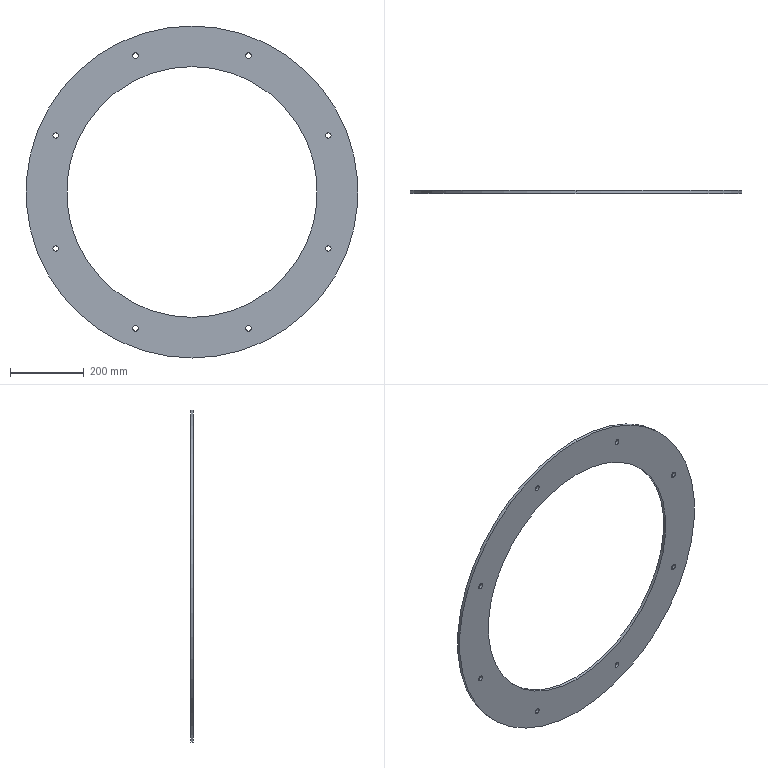Part | SolidWorks | features Extrusion 1, HoleWzd 1 | 1 solid | 22 faces | box 900 x 8 x 900 mm | volume 2172725 mm3 | cylinder 20 | plane 2 | commonest cylinder face diameters 15 x16 680 x2 900 x2
STEP:
#1=CARTESIAN_POINT('',(153.073,-4.,-377.052));
#2=VERTEX_POINT('',#1);
#3=CARTESIAN_POINT('',(153.073,-4.,-362.052));
#4=VERTEX_POINT('',#3);
#5=CARTESIAN_POINT('',(153.073,-4.,-369.552));
#6=DIRECTION('',(0.,1.,0.));
#7=DIRECTION('',(0.,0.,1.));
#8=AXIS2_PLACEMENT_3D('',#5,#6,#7);
#9=CIRCLE('',#8,7.5);
#10=EDGE_CURVE('',#2,#4,#9,.T.);
#11=ORIENTED_EDGE('',*,*,#10,.F.);
#12=CARTESIAN_POINT('',(153.073,4.,-377.052));
#13=VERTEX_POINT('',#12);
#14=CARTESIAN_POINT('',(153.073,4.,-377.052));
#15=DIRECTION('',(0.,1.,0.));
#16=VECTOR('',#15,1000.);
#17=LINE('',#14,#16);
#18=EDGE_CURVE('',#2,#13,#17,.T.);
#19=ORIENTED_EDGE('',*,*,#18,.T.);
#20=CARTESIAN_POINT('',(153.073,4.,-362.052));
#21=VERTEX_POINT('',#20);
#22=CARTESIAN_POINT('',(153.073,4.,-369.552));
#23=DIRECTION('',(0.,1.,0.));
#24=DIRECTION('',(0.,0.,1.));
#25=AXIS2_PLACEMENT_3D('',#22,#23,#24);
#26=CIRCLE('',#25,7.5);
#27=EDGE_CURVE('',#13,#21,#26,.T.);
#28=ORIENTED_EDGE('',*,*,#27,.T.);
#29=CARTESIAN_POINT('',(153.073,4.,-362.052));
#30=DIRECTION('',(0.,1.,0.));
#31=VECTOR('',#30,1000.);
#32=LINE('',#29,#31);
#33=EDGE_CURVE('',#4,#21,#32,.T.);
#34=ORIENTED_EDGE('',*,*,#33,.F.);
#35=EDGE_LOOP('',(#11,#19,#28,#34));
#36=FACE_OUTER_BOUND('',#35,.T.);
#37=CARTESIAN_POINT('',(153.073,4.,-369.552));
#38=DIRECTION('',(0.,1.,0.));
#39=DIRECTION('',(0.,0.,1.));
#40=AXIS2_PLACEMENT_3D('',#37,#38,#39);
#41=CYLINDRICAL_SURFACE('',#40,7.5);
#42=ADVANCED_FACE('',(#36),#41,.F.);
#43=CARTESIAN_POINT('',(369.552,-4.,-160.573));
#44=VERTEX_POINT('',#43);
#45=CARTESIAN_POINT('',(369.552,-4.,-145.573));
#46=VERTEX_POINT('',#45);
#47=CARTESIAN_POINT('',(369.552,-4.,-153.073));
#48=DIRECTION('',(0.,1.,0.));
#49=DIRECTION('',(0.,0.,1.));
#50=AXIS2_PLACEMENT_3D('',#47,#48,#49);
#51=CIRCLE('',#50,7.5);
#52=EDGE_CURVE('',#44,#46,#51,.T.);
#53=ORIENTED_EDGE('',*,*,#52,.F.);
#54=CARTESIAN_POINT('',(369.552,4.,-160.573));
#55=VERTEX_POINT('',#54);
#56=CARTESIAN_POINT('',(369.552,4.,-160.573));
#57=DIRECTION('',(0.,1.,0.));
#58=VECTOR('',#57,1000.);
#59=LINE('',#56,#58);
#60=EDGE_CURVE('',#44,#55,#59,.T.);
#61=ORIENTED_EDGE('',*,*,#60,.T.);
#62=CARTESIAN_POINT('',(369.552,4.,-145.573));
#63=VERTEX_POINT('',#62);
#64=CARTESIAN_POINT('',(369.552,4.,-153.073));
#65=DIRECTION('',(0.,1.,0.));
#66=DIRECTION('',(0.,0.,1.));
#67=AXIS2_PLACEMENT_3D('',#64,#65,#66);
#68=CIRCLE('',#67,7.5);
#69=EDGE_CURVE('',#55,#63,#68,.T.);
#70=ORIENTED_EDGE('',*,*,#69,.T.);
#71=CARTESIAN_POINT('',(369.552,4.,-145.573));
#72=DIRECTION('',(0.,1.,0.));
#73=VECTOR('',#72,1000.);
#74=LINE('',#71,#73);
#75=EDGE_CURVE('',#46,#63,#74,.T.);
#76=ORIENTED_EDGE('',*,*,#75,.F.);
#77=EDGE_LOOP('',(#53,#61,#70,#76));
#78=FACE_OUTER_BOUND('',#77,.T.);
#79=CARTESIAN_POINT('',(369.552,4.,-153.073));
#80=DIRECTION('',(0.,1.,0.));
#81=DIRECTION('',(0.,0.,1.));
#82=AXIS2_PLACEMENT_3D('',#79,#80,#81);
#83=CYLINDRICAL_SURFACE('',#82,7.5);
#84=ADVANCED_FACE('',(#78),#83,.F.);
#85=CARTESIAN_POINT('',(369.552,-4.,145.573));
#86=VERTEX_POINT('',#85);
#87=CARTESIAN_POINT('',(369.552,-4.,160.573));
#88=VERTEX_POINT('',#87);
#89=CARTESIAN_POINT('',(369.552,-4.,153.073));
#90=DIRECTION('',(0.,1.,0.));
#91=DIRECTION('',(0.,0.,1.));
#92=AXIS2_PLACEMENT_3D('',#89,#90,#91);
#93=CIRCLE('',#92,7.5);
#94=EDGE_CURVE('',#86,#88,#93,.T.);
#95=ORIENTED_EDGE('',*,*,#94,.F.);
#96=CARTESIAN_POINT('',(369.552,4.,145.573));
#97=VERTEX_POINT('',#96);
#98=CARTESIAN_POINT('',(369.552,4.,145.573));
#99=DIRECTION('',(0.,1.,0.));
#100=VECTOR('',#99,1000.);
#101=LINE('',#98,#100);
#102=EDGE_CURVE('',#86,#97,#101,.T.);
#103=ORIENTED_EDGE('',*,*,#102,.T.);
#104=CARTESIAN_POINT('',(369.552,4.,160.573));
#105=VERTEX_POINT('',#104);
#106=CARTESIAN_POINT('',(369.552,4.,153.073));
#107=DIRECTION('',(0.,1.,0.));
#108=DIRECTION('',(0.,0.,1.));
#109=AXIS2_PLACEMENT_3D('',#106,#107,#108);
#110=CIRCLE('',#109,7.5);
#111=EDGE_CURVE('',#97,#105,#110,.T.);
#112=ORIENTED_EDGE('',*,*,#111,.T.);
#113=CARTESIAN_POINT('',(369.552,4.,160.573));
#114=DIRECTION('',(0.,1.,0.));
#115=VECTOR('',#114,1000.);
#116=LINE('',#113,#115);
#117=EDGE_CURVE('',#88,#105,#116,.T.);
#118=ORIENTED_EDGE('',*,*,#117,.F.);
#119=EDGE_LOOP('',(#95,#103,#112,#118));
#120=FACE_OUTER_BOUND('',#119,.T.);
#121=CARTESIAN_POINT('',(369.552,4.,153.073));
#122=DIRECTION('',(0.,1.,0.));
#123=DIRECTION('',(0.,0.,1.));
#124=AXIS2_PLACEMENT_3D('',#121,#122,#123);
#125=CYLINDRICAL_SURFACE('',#124,7.5);
#126=ADVANCED_FACE('',(#120),#125,.F.);
#127=CARTESIAN_POINT('',(153.073,-4.,362.052));
#128=VERTEX_POINT('',#127);
#129=CARTESIAN_POINT('',(153.073,-4.,377.052));
#130=VERTEX_POINT('',#129);
#131=CARTESIAN_POINT('',(153.073,-4.,369.552));
#132=DIRECTION('',(0.,1.,0.));
#133=DIRECTION('',(0.,0.,1.));
#134=AXIS2_PLACEMENT_3D('',#131,#132,#133);
#135=CIRCLE('',#134,7.5);
#136=EDGE_CURVE('',#128,#130,#135,.T.);
#137=ORIENTED_EDGE('',*,*,#136,.F.);
#138=CARTESIAN_POINT('',(153.073,4.,362.052));
#139=VERTEX_POINT('',#138);
#140=CARTESIAN_POINT('',(153.073,4.,362.052));
#141=DIRECTION('',(0.,1.,0.));
#142=VECTOR('',#141,1000.);
#143=LINE('',#140,#142);
#144=EDGE_CURVE('',#128,#139,#143,.T.);
#145=ORIENTED_EDGE('',*,*,#144,.T.);
#146=CARTESIAN_POINT('',(153.073,4.,377.052));
#147=VERTEX_POINT('',#146);
#148=CARTESIAN_POINT('',(153.073,4.,369.552));
#149=DIRECTION('',(0.,1.,0.));
#150=DIRECTION('',(0.,0.,1.));
#151=AXIS2_PLACEMENT_3D('',#148,#149,#150);
#152=CIRCLE('',#151,7.5);
#153=EDGE_CURVE('',#139,#147,#152,.T.);
#154=ORIENTED_EDGE('',*,*,#153,.T.);
#155=CARTESIAN_POINT('',(153.073,4.,377.052));
#156=DIRECTION('',(0.,1.,0.));
#157=VECTOR('',#156,1000.);
#158=LINE('',#155,#157);
#159=EDGE_CURVE('',#130,#147,#158,.T.);
#160=ORIENTED_EDGE('',*,*,#159,.F.);
#161=EDGE_LOOP('',(#137,#145,#154,#160));
#162=FACE_OUTER_BOUND('',#161,.T.);
#163=CARTESIAN_POINT('',(153.073,4.,369.552));
#164=DIRECTION('',(0.,1.,0.));
#165=DIRECTION('',(0.,0.,1.));
#166=AXIS2_PLACEMENT_3D('',#163,#164,#165);
#167=CYLINDRICAL_SURFACE('',#166,7.5);
#168=ADVANCED_FACE('',(#162),#167,.F.);
#169=CARTESIAN_POINT('',(-153.073,-4.,362.052));
#170=VERTEX_POINT('',#169);
#171=CARTESIAN_POINT('',(-153.073,-4.,377.052));
#172=VERTEX_POINT('',#171);
#173=CARTESIAN_POINT('',(-153.073,-4.,369.552));
#174=DIRECTION('',(0.,1.,0.));
#175=DIRECTION('',(0.,0.,1.));
#176=AXIS2_PLACEMENT_3D('',#173,#174,#175);
#177=CIRCLE('',#176,7.5);
#178=EDGE_CURVE('',#170,#172,#177,.T.);
#179=ORIENTED_EDGE('',*,*,#178,.F.);
#180=CARTESIAN_POINT('',(-153.073,4.,362.052));
#181=VERTEX_POINT('',#180);
#182=CARTESIAN_POINT('',(-153.073,4.,362.052));
#183=DIRECTION('',(0.,1.,0.));
#184=VECTOR('',#183,1000.);
#185=LINE('',#182,#184);
#186=EDGE_CURVE('',#170,#181,#185,.T.);
#187=ORIENTED_EDGE('',*,*,#186,.T.);
#188=CARTESIAN_POINT('',(-153.073,4.,377.052));
#189=VERTEX_POINT('',#188);
#190=CARTESIAN_POINT('',(-153.073,4.,369.552));
#191=DIRECTION('',(0.,1.,0.));
#192=DIRECTION('',(0.,0.,1.));
#193=AXIS2_PLACEMENT_3D('',#190,#191,#192);
#194=CIRCLE('',#193,7.5);
#195=EDGE_CURVE('',#181,#189,#194,.T.);
#196=ORIENTED_EDGE('',*,*,#195,.T.);
#197=CARTESIAN_POINT('',(-153.073,4.,377.052));
#198=DIRECTION('',(0.,1.,0.));
#199=VECTOR('',#198,1000.);
#200=LINE('',#197,#199);
#201=EDGE_CURVE('',#172,#189,#200,.T.);
#202=ORIENTED_EDGE('',*,*,#201,.F.);
#203=EDGE_LOOP('',(#179,#187,#196,#202));
#204=FACE_OUTER_BOUND('',#203,.T.);
#205=CARTESIAN_POINT('',(-153.073,4.,369.552));
#206=DIRECTION('',(0.,1.,0.));
#207=DIRECTION('',(0.,0.,1.));
#208=AXIS2_PLACEMENT_3D('',#205,#206,#207);
#209=CYLINDRICAL_SURFACE('',#208,7.5);
#210=ADVANCED_FACE('',(#204),#209,.F.);
#211=CARTESIAN_POINT('',(-369.552,-4.,145.573));
#212=VERTEX_POINT('',#211);
#213=CARTESIAN_POINT('',(-369.552,-4.,160.573));
#214=VERTEX_POINT('',#213);
#215=CARTESIAN_POINT('',(-369.552,-4.,153.073));
#216=DIRECTION('',(0.,1.,0.));
#217=DIRECTION('',(0.,0.,1.));
#218=AXIS2_PLACEMENT_3D('',#215,#216,#217);
#219=CIRCLE('',#218,7.5);
#220=EDGE_CURVE('',#212,#214,#219,.T.);
#221=ORIENTED_EDGE('',*,*,#220,.F.);
#222=CARTESIAN_POINT('',(-369.552,4.,145.573));
#223=VERTEX_POINT('',#222);
#224=CARTESIAN_POINT('',(-369.552,4.,145.573));
#225=DIRECTION('',(0.,1.,0.));
#226=VECTOR('',#225,1000.);
#227=LINE('',#224,#226);
#228=EDGE_CURVE('',#212,#223,#227,.T.);
#229=ORIENTED_EDGE('',*,*,#228,.T.);
#230=CARTESIAN_POINT('',(-369.552,4.,160.573));
#231=VERTEX_POINT('',#230);
#232=CARTESIAN_POINT('',(-369.552,4.,153.073));
#233=DIRECTION('',(0.,1.,0.));
#234=DIRECTION('',(0.,0.,1.));
#235=AXIS2_PLACEMENT_3D('',#232,#233,#234);
#236=CIRCLE('',#235,7.5);
#237=EDGE_CURVE('',#223,#231,#236,.T.);
#238=ORIENTED_EDGE('',*,*,#237,.T.);
#239=CARTESIAN_POINT('',(-369.552,4.,160.573));
#240=DIRECTION('',(0.,1.,0.));
#241=VECTOR('',#240,1000.);
#242=LINE('',#239,#241);
#243=EDGE_CURVE('',#214,#231,#242,.T.);
#244=ORIENTED_EDGE('',*,*,#243,.F.);
#245=EDGE_LOOP('',(#221,#229,#238,#244));
#246=FACE_OUTER_BOUND('',#245,.T.);
#247=CARTESIAN_POINT('',(-369.552,4.,153.073));
#248=DIRECTION('',(0.,1.,0.));
#249=DIRECTION('',(0.,0.,1.));
#250=AXIS2_PLACEMENT_3D('',#247,#248,#249);
#251=CYLINDRICAL_SURFACE('',#250,7.5);
#252=ADVANCED_FACE('',(#246),#251,.F.);
#253=CARTESIAN_POINT('',(-369.552,-4.,-160.573));
#254=VERTEX_POINT('',#253);
#255=CARTESIAN_POINT('',(-369.552,-4.,-145.573));
#256=VERTEX_POINT('',#255);
#257=CARTESIAN_POINT('',(-369.552,-4.,-153.073));
#258=DIRECTION('',(0.,1.,0.));
#259=DIRECTION('',(0.,0.,1.));
#260=AXIS2_PLACEMENT_3D('',#257,#258,#259);
#261=CIRCLE('',#260,7.5);
#262=EDGE_CURVE('',#254,#256,#261,.T.);
#263=ORIENTED_EDGE('',*,*,#262,.F.);
#264=CARTESIAN_POINT('',(-369.552,4.,-160.573));
#265=VERTEX_POINT('',#264);
#266=CARTESIAN_POINT('',(-369.552,4.,-160.573));
#267=DIRECTION('',(0.,1.,0.));
#268=VECTOR('',#267,1000.);
#269=LINE('',#266,#268);
#270=EDGE_CURVE('',#254,#265,#269,.T.);
#271=ORIENTED_EDGE('',*,*,#270,.T.);
#272=CARTESIAN_POINT('',(-369.552,4.,-145.573));
#273=VERTEX_POINT('',#272);
#274=CARTESIAN_POINT('',(-369.552,4.,-153.073));
#275=DIRECTION('',(0.,1.,0.));
#276=DIRECTION('',(0.,0.,1.));
#277=AXIS2_PLACEMENT_3D('',#274,#275,#276);
#278=CIRCLE('',#277,7.5);
#279=EDGE_CURVE('',#265,#273,#278,.T.);
#280=ORIENTED_EDGE('',*,*,#279,.T.);
#281=CARTESIAN_POINT('',(-369.552,4.,-145.573));
#282=DIRECTION('',(0.,1.,0.));
#283=VECTOR('',#282,1000.);
#284=LINE('',#281,#283);
#285=EDGE_CURVE('',#256,#273,#284,.T.);
#286=ORIENTED_EDGE('',*,*,#285,.F.);
#287=EDGE_LOOP('',(#263,#271,#280,#286));
#288=FACE_OUTER_BOUND('',#287,.T.);
#289=CARTESIAN_POINT('',(-369.552,4.,-153.073));
#290=DIRECTION('',(0.,1.,0.));
#291=DIRECTION('',(0.,0.,1.));
#292=AXIS2_PLACEMENT_3D('',#289,#290,#291);
#293=CYLINDRICAL_SURFACE('',#292,7.5);
#294=ADVANCED_FACE('',(#288),#293,.F.);
#295=CARTESIAN_POINT('',(-153.073,-4.,-377.052));
#296=VERTEX_POINT('',#295);
#297=CARTESIAN_POINT('',(-153.073,-4.,-362.052));
#298=VERTEX_POINT('',#297);
#299=CARTESIAN_POINT('',(-153.073,-4.,-369.552));
#300=DIRECTION('',(0.,1.,0.));
#301=DIRECTION('',(0.,0.,1.));
#302=AXIS2_PLACEMENT_3D('',#299,#300,#301);
#303=CIRCLE('',#302,7.5);
#304=EDGE_CURVE('',#296,#298,#303,.T.);
#305=ORIENTED_EDGE('',*,*,#304,.F.);
#306=CARTESIAN_POINT('',(-153.073,4.,-377.052));
#307=VERTEX_POINT('',#306);
#308=CARTESIAN_POINT('',(-153.073,4.,-377.052));
#309=DIRECTION('',(0.,1.,0.));
#310=VECTOR('',#309,1000.);
#311=LINE('',#308,#310);
#312=EDGE_CURVE('',#296,#307,#311,.T.);
#313=ORIENTED_EDGE('',*,*,#312,.T.);
#314=CARTESIAN_POINT('',(-153.073,4.,-362.052));
#315=VERTEX_POINT('',#314);
#316=CARTESIAN_POINT('',(-153.073,4.,-369.552));
#317=DIRECTION('',(0.,1.,0.));
#318=DIRECTION('',(0.,0.,1.));
#319=AXIS2_PLACEMENT_3D('',#316,#317,#318);
#320=CIRCLE('',#319,7.5);
#321=EDGE_CURVE('',#307,#315,#320,.T.);
#322=ORIENTED_EDGE('',*,*,#321,.T.);
#323=CARTESIAN_POINT('',(-153.073,4.,-362.052));
#324=DIRECTION('',(0.,1.,0.));
#325=VECTOR('',#324,1000.);
#326=LINE('',#323,#325);
#327=EDGE_CURVE('',#298,#315,#326,.T.);
#328=ORIENTED_EDGE('',*,*,#327,.F.);
#329=EDGE_LOOP('',(#305,#313,#322,#328));
#330=FACE_OUTER_BOUND('',#329,.T.);
#331=CARTESIAN_POINT('',(-153.073,4.,-369.552));
#332=DIRECTION('',(0.,1.,0.));
#333=DIRECTION('',(0.,0.,1.));
#334=AXIS2_PLACEMENT_3D('',#331,#332,#333);
#335=CYLINDRICAL_SURFACE('',#334,7.5);
#336=ADVANCED_FACE('',(#330),#335,.F.);
#337=CARTESIAN_POINT('',(0.,4.,-340.));
#338=VERTEX_POINT('',#337);
#339=CARTESIAN_POINT('',(0.,4.,340.));
#340=VERTEX_POINT('',#339);
#341=CARTESIAN_POINT('',(0.,4.,0.));
#342=DIRECTION('',(0.,1.,0.));
#343=DIRECTION('',(0.,0.,1.));
#344=AXIS2_PLACEMENT_3D('',#341,#342,#343);
#345=CIRCLE('',#344,340.);
#346=EDGE_CURVE('',#338,#340,#345,.T.);
#347=ORIENTED_EDGE('',*,*,#346,.T.);
#348=CARTESIAN_POINT('',(0.,-4.,340.));
#349=VERTEX_POINT('',#348);
#350=CARTESIAN_POINT('',(0.,4.,340.));
#351=DIRECTION('',(0.,-1.,0.));
#352=VECTOR('',#351,1000.);
#353=LINE('',#350,#352);
#354=EDGE_CURVE('',#340,#349,#353,.T.);
#355=ORIENTED_EDGE('',*,*,#354,.T.);
#356=CARTESIAN_POINT('',(0.,-4.,-340.));
#357=VERTEX_POINT('',#356);
#358=CARTESIAN_POINT('',(0.,-4.,0.));
#359=DIRECTION('',(0.,1.,0.));
#360=DIRECTION('',(0.,0.,1.));
#361=AXIS2_PLACEMENT_3D('',#358,#359,#360);
#362=CIRCLE('',#361,340.);
#363=EDGE_CURVE('',#357,#349,#362,.T.);
#364=ORIENTED_EDGE('',*,*,#363,.F.);
#365=CARTESIAN_POINT('',(0.,4.,-340.));
#366=DIRECTION('',(0.,-1.,0.));
#367=VECTOR('',#366,1000.);
#368=LINE('',#365,#367);
#369=EDGE_CURVE('',#338,#357,#368,.T.);
#370=ORIENTED_EDGE('',*,*,#369,.F.);
#371=EDGE_LOOP('',(#347,#355,#364,#370));
#372=FACE_OUTER_BOUND('',#371,.T.);
#373=CARTESIAN_POINT('',(0.,4.,0.));
#374=DIRECTION('',(0.,-1.,0.));
#375=DIRECTION('',(0.,0.,-1.));
#376=AXIS2_PLACEMENT_3D('',#373,#374,#375);
#377=CYLINDRICAL_SURFACE('',#376,340.);
#378=ADVANCED_FACE('',(#372),#377,.F.);
#379=CARTESIAN_POINT('',(0.,4.,450.));
#380=VERTEX_POINT('',#379);
#381=CARTESIAN_POINT('',(0.,4.,-450.));
#382=VERTEX_POINT('',#381);
#383=CARTESIAN_POINT('',(0.,4.,0.));
#384=DIRECTION('',(0.,1.,0.));
#385=DIRECTION('',(0.,0.,1.));
#386=AXIS2_PLACEMENT_3D('',#383,#384,#385);
#387=CIRCLE('',#386,450.);
#388=EDGE_CURVE('',#380,#382,#387,.T.);
#389=ORIENTED_EDGE('',*,*,#388,.F.);
#390=CARTESIAN_POINT('',(0.,-4.,450.));
#391=VERTEX_POINT('',#390);
#392=CARTESIAN_POINT('',(0.,4.,450.));
#393=DIRECTION('',(0.,-1.,0.));
#394=VECTOR('',#393,1000.);
#395=LINE('',#392,#394);
#396=EDGE_CURVE('',#380,#391,#395,.T.);
#397=ORIENTED_EDGE('',*,*,#396,.T.);
#398=CARTESIAN_POINT('',(0.,-4.,-450.));
#399=VERTEX_POINT('',#398);
#400=CARTESIAN_POINT('',(0.,-4.,0.));
#401=DIRECTION('',(0.,1.,0.));
#402=DIRECTION('',(0.,0.,1.));
#403=AXIS2_PLACEMENT_3D('',#400,#401,#402);
#404=CIRCLE('',#403,450.);
#405=EDGE_CURVE('',#391,#399,#404,.T.);
#406=ORIENTED_EDGE('',*,*,#405,.T.);
#407=CARTESIAN_POINT('',(0.,4.,-450.));
#408=DIRECTION('',(0.,-1.,0.));
#409=VECTOR('',#408,1000.);
#410=LINE('',#407,#409);
#411=EDGE_CURVE('',#382,#399,#410,.T.);
#412=ORIENTED_EDGE('',*,*,#411,.F.);
#413=EDGE_LOOP('',(#389,#397,#406,#412));
#414=FACE_OUTER_BOUND('',#413,.T.);
#415=CARTESIAN_POINT('',(0.,4.,0.));
#416=DIRECTION('',(0.,-1.,0.));
#417=DIRECTION('',(0.,0.,-1.));
#418=AXIS2_PLACEMENT_3D('',#415,#416,#417);
#419=CYLINDRICAL_SURFACE('',#418,450.);
#420=ADVANCED_FACE('',(#414),#419,.T.);
#421=CARTESIAN_POINT('',(153.073,4.,-369.552));
#422=DIRECTION('',(0.,1.,0.));
#423=DIRECTION('',(0.,0.,1.));
#424=AXIS2_PLACEMENT_3D('',#421,#422,#423);
#425=CIRCLE('',#424,7.5);
#426=EDGE_CURVE('',#21,#13,#425,.T.);
#427=ORIENTED_EDGE('',*,*,#426,.F.);
#428=ORIENTED_EDGE('',*,*,#27,.F.);
#429=EDGE_LOOP('',(#427,#428));
#430=FACE_BOUND('',#429,.T.);
#431=CARTESIAN_POINT('',(369.552,4.,-153.073));
#432=DIRECTION('',(0.,1.,0.));
#433=DIRECTION('',(0.,0.,1.));
#434=AXIS2_PLACEMENT_3D('',#431,#432,#433);
#435=CIRCLE('',#434,7.5);
#436=EDGE_CURVE('',#63,#55,#435,.T.);
#437=ORIENTED_EDGE('',*,*,#436,.F.);
#438=ORIENTED_EDGE('',*,*,#69,.F.);
#439=EDGE_LOOP('',(#437,#438));
#440=FACE_BOUND('',#439,.T.);
#441=CARTESIAN_POINT('',(369.552,4.,153.073));
#442=DIRECTION('',(0.,1.,0.));
#443=DIRECTION('',(0.,0.,1.));
#444=AXIS2_PLACEMENT_3D('',#441,#442,#443);
#445=CIRCLE('',#444,7.5);
#446=EDGE_CURVE('',#105,#97,#445,.T.);
#447=ORIENTED_EDGE('',*,*,#446,.F.);
#448=ORIENTED_EDGE('',*,*,#111,.F.);
#449=EDGE_LOOP('',(#447,#448));
#450=FACE_BOUND('',#449,.T.);
#451=CARTESIAN_POINT('',(153.073,4.,369.552));
#452=DIRECTION('',(0.,1.,0.));
#453=DIRECTION('',(0.,0.,1.));
#454=AXIS2_PLACEMENT_3D('',#451,#452,#453);
#455=CIRCLE('',#454,7.5);
#456=EDGE_CURVE('',#147,#139,#455,.T.);
#457=ORIENTED_EDGE('',*,*,#456,.F.);
#458=ORIENTED_EDGE('',*,*,#153,.F.);
#459=EDGE_LOOP('',(#457,#458));
#460=FACE_BOUND('',#459,.T.);
#461=CARTESIAN_POINT('',(-153.073,4.,369.552));
#462=DIRECTION('',(0.,1.,0.));
#463=DIRECTION('',(0.,0.,1.));
#464=AXIS2_PLACEMENT_3D('',#461,#462,#463);
#465=CIRCLE('',#464,7.5);
#466=EDGE_CURVE('',#189,#181,#465,.T.);
#467=ORIENTED_EDGE('',*,*,#466,.F.);
#468=ORIENTED_EDGE('',*,*,#195,.F.);
#469=EDGE_LOOP('',(#467,#468));
#470=FACE_BOUND('',#469,.T.);
#471=CARTESIAN_POINT('',(-369.552,4.,153.073));
#472=DIRECTION('',(0.,1.,0.));
#473=DIRECTION('',(0.,0.,1.));
#474=AXIS2_PLACEMENT_3D('',#471,#472,#473);
#475=CIRCLE('',#474,7.5);
#476=EDGE_CURVE('',#231,#223,#475,.T.);
#477=ORIENTED_EDGE('',*,*,#476,.F.);
#478=ORIENTED_EDGE('',*,*,#237,.F.);
#479=EDGE_LOOP('',(#477,#478));
#480=FACE_BOUND('',#479,.T.);
#481=CARTESIAN_POINT('',(-369.552,4.,-153.073));
#482=DIRECTION('',(0.,1.,0.));
#483=DIRECTION('',(0.,0.,1.));
#484=AXIS2_PLACEMENT_3D('',#481,#482,#483);
#485=CIRCLE('',#484,7.5);
#486=EDGE_CURVE('',#273,#265,#485,.T.);
#487=ORIENTED_EDGE('',*,*,#486,.F.);
#488=ORIENTED_EDGE('',*,*,#279,.F.);
#489=EDGE_LOOP('',(#487,#488));
#490=FACE_BOUND('',#489,.T.);
#491=CARTESIAN_POINT('',(-153.073,4.,-369.552));
#492=DIRECTION('',(0.,1.,0.));
#493=DIRECTION('',(0.,0.,1.));
#494=AXIS2_PLACEMENT_3D('',#491,#492,#493);
#495=CIRCLE('',#494,7.5);
#496=EDGE_CURVE('',#315,#307,#495,.T.);
#497=ORIENTED_EDGE('',*,*,#496,.F.);
#498=ORIENTED_EDGE('',*,*,#321,.F.);
#499=EDGE_LOOP('',(#497,#498));
#500=FACE_BOUND('',#499,.T.);
#501=CARTESIAN_POINT('',(0.,4.,0.));
#502=DIRECTION('',(0.,1.,0.));
#503=DIRECTION('',(0.,0.,1.));
#504=AXIS2_PLACEMENT_3D('',#501,#502,#503);
#505=CIRCLE('',#504,450.);
#506=EDGE_CURVE('',#382,#380,#505,.T.);
#507=ORIENTED_EDGE('',*,*,#506,.T.);
#508=ORIENTED_EDGE('',*,*,#388,.T.);
#509=EDGE_LOOP('',(#507,#508));
#510=FACE_OUTER_BOUND('',#509,.T.);
#511=ORIENTED_EDGE('',*,*,#346,.F.);
#512=CARTESIAN_POINT('',(0.,4.,0.));
#513=DIRECTION('',(0.,1.,0.));
#514=DIRECTION('',(0.,0.,1.));
#515=AXIS2_PLACEMENT_3D('',#512,#513,#514);
#516=CIRCLE('',#515,340.);
#517=EDGE_CURVE('',#340,#338,#516,.T.);
#518=ORIENTED_EDGE('',*,*,#517,.F.);
#519=EDGE_LOOP('',(#511,#518));
#520=FACE_BOUND('',#519,.T.);
#521=CARTESIAN_POINT('',(0.,4.,0.));
#522=DIRECTION('',(0.,1.,0.));
#523=DIRECTION('',(0.,0.,1.));
#524=AXIS2_PLACEMENT_3D('',#521,#522,#523);
#525=PLANE('',#524);
#526=ADVANCED_FACE('',(#430,#440,#450,#460,#470,#480,#490,#500,#510,#520),#525,.T.);
#527=CARTESIAN_POINT('',(153.073,-4.,-369.552));
#528=DIRECTION('',(0.,1.,0.));
#529=DIRECTION('',(0.,0.,1.));
#530=AXIS2_PLACEMENT_3D('',#527,#528,#529);
#531=CIRCLE('',#530,7.5);
#532=EDGE_CURVE('',#4,#2,#531,.T.);
#533=ORIENTED_EDGE('',*,*,#532,.T.);
#534=ORIENTED_EDGE('',*,*,#10,.T.);
#535=EDGE_LOOP('',(#533,#534));
#536=FACE_BOUND('',#535,.T.);
#537=CARTESIAN_POINT('',(369.552,-4.,-153.073));
#538=DIRECTION('',(0.,1.,0.));
#539=DIRECTION('',(0.,0.,1.));
#540=AXIS2_PLACEMENT_3D('',#537,#538,#539);
#541=CIRCLE('',#540,7.5);
#542=EDGE_CURVE('',#46,#44,#541,.T.);
#543=ORIENTED_EDGE('',*,*,#542,.T.);
#544=ORIENTED_EDGE('',*,*,#52,.T.);
#545=EDGE_LOOP('',(#543,#544));
#546=FACE_BOUND('',#545,.T.);
#547=CARTESIAN_POINT('',(369.552,-4.,153.073));
#548=DIRECTION('',(0.,1.,0.));
#549=DIRECTION('',(0.,0.,1.));
#550=AXIS2_PLACEMENT_3D('',#547,#548,#549);
#551=CIRCLE('',#550,7.5);
#552=EDGE_CURVE('',#88,#86,#551,.T.);
#553=ORIENTED_EDGE('',*,*,#552,.T.);
#554=ORIENTED_EDGE('',*,*,#94,.T.);
#555=EDGE_LOOP('',(#553,#554));
#556=FACE_BOUND('',#555,.T.);
#557=CARTESIAN_POINT('',(153.073,-4.,369.552));
#558=DIRECTION('',(0.,1.,0.));
#559=DIRECTION('',(0.,0.,1.));
#560=AXIS2_PLACEMENT_3D('',#557,#558,#559);
#561=CIRCLE('',#560,7.5);
#562=EDGE_CURVE('',#130,#128,#561,.T.);
#563=ORIENTED_EDGE('',*,*,#562,.T.);
#564=ORIENTED_EDGE('',*,*,#136,.T.);
#565=EDGE_LOOP('',(#563,#564));
#566=FACE_BOUND('',#565,.T.);
#567=CARTESIAN_POINT('',(-153.073,-4.,369.552));
#568=DIRECTION('',(0.,1.,0.));
#569=DIRECTION('',(0.,0.,1.));
#570=AXIS2_PLACEMENT_3D('',#567,#568,#569);
#571=CIRCLE('',#570,7.5);
#572=EDGE_CURVE('',#172,#170,#571,.T.);
#573=ORIENTED_EDGE('',*,*,#572,.T.);
#574=ORIENTED_EDGE('',*,*,#178,.T.);
#575=EDGE_LOOP('',(#573,#574));
#576=FACE_BOUND('',#575,.T.);
#577=CARTESIAN_POINT('',(-369.552,-4.,153.073));
#578=DIRECTION('',(0.,1.,0.));
#579=DIRECTION('',(0.,0.,1.));
#580=AXIS2_PLACEMENT_3D('',#577,#578,#579);
#581=CIRCLE('',#580,7.5);
#582=EDGE_CURVE('',#214,#212,#581,.T.);
#583=ORIENTED_EDGE('',*,*,#582,.T.);
#584=ORIENTED_EDGE('',*,*,#220,.T.);
#585=EDGE_LOOP('',(#583,#584));
#586=FACE_BOUND('',#585,.T.);
#587=CARTESIAN_POINT('',(-369.552,-4.,-153.073));
#588=DIRECTION('',(0.,1.,0.));
#589=DIRECTION('',(0.,0.,1.));
#590=AXIS2_PLACEMENT_3D('',#587,#588,#589);
#591=CIRCLE('',#590,7.5);
#592=EDGE_CURVE('',#256,#254,#591,.T.);
#593=ORIENTED_EDGE('',*,*,#592,.T.);
#594=ORIENTED_EDGE('',*,*,#262,.T.);
#595=EDGE_LOOP('',(#593,#594));
#596=FACE_BOUND('',#595,.T.);
#597=CARTESIAN_POINT('',(-153.073,-4.,-369.552));
#598=DIRECTION('',(0.,1.,0.));
#599=DIRECTION('',(0.,0.,1.));
#600=AXIS2_PLACEMENT_3D('',#597,#598,#599);
#601=CIRCLE('',#600,7.5);
#602=EDGE_CURVE('',#298,#296,#601,.T.);
#603=ORIENTED_EDGE('',*,*,#602,.T.);
#604=ORIENTED_EDGE('',*,*,#304,.T.);
#605=EDGE_LOOP('',(#603,#604));
#606=FACE_BOUND('',#605,.T.);
#607=CARTESIAN_POINT('',(0.,-4.,0.));
#608=DIRECTION('',(0.,1.,0.));
#609=DIRECTION('',(0.,0.,1.));
#610=AXIS2_PLACEMENT_3D('',#607,#608,#609);
#611=CIRCLE('',#610,450.);
#612=EDGE_CURVE('',#399,#391,#611,.T.);
#613=ORIENTED_EDGE('',*,*,#612,.F.);
#614=ORIENTED_EDGE('',*,*,#405,.F.);
#615=EDGE_LOOP('',(#613,#614));
#616=FACE_OUTER_BOUND('',#615,.T.);
#617=ORIENTED_EDGE('',*,*,#363,.T.);
#618=CARTESIAN_POINT('',(0.,-4.,0.));
#619=DIRECTION('',(0.,1.,0.));
#620=DIRECTION('',(0.,0.,1.));
#621=AXIS2_PLACEMENT_3D('',#618,#619,#620);
#622=CIRCLE('',#621,340.);
#623=EDGE_CURVE('',#349,#357,#622,.T.);
#624=ORIENTED_EDGE('',*,*,#623,.T.);
#625=EDGE_LOOP('',(#617,#624));
#626=FACE_BOUND('',#625,.T.);
#627=CARTESIAN_POINT('',(0.,-4.,0.));
#628=DIRECTION('',(0.,1.,0.));
#629=DIRECTION('',(0.,0.,1.));
#630=AXIS2_PLACEMENT_3D('',#627,#628,#629);
#631=PLANE('',#630);
#632=ADVANCED_FACE('',(#536,#546,#556,#566,#576,#586,#596,#606,#616,#626),#631,.F.);
#633=ORIENTED_EDGE('',*,*,#396,.F.);
#634=ORIENTED_EDGE('',*,*,#506,.F.);
#635=ORIENTED_EDGE('',*,*,#411,.T.);
#636=ORIENTED_EDGE('',*,*,#612,.T.);
#637=EDGE_LOOP('',(#633,#634,#635,#636));
#638=FACE_OUTER_BOUND('',#637,.T.);
#639=CARTESIAN_POINT('',(0.,4.,0.));
#640=DIRECTION('',(0.,-1.,0.));
#641=DIRECTION('',(0.,0.,-1.));
#642=AXIS2_PLACEMENT_3D('',#639,#640,#641);
#643=CYLINDRICAL_SURFACE('',#642,450.);
#644=ADVANCED_FACE('',(#638),#643,.T.);
#645=ORIENTED_EDGE('',*,*,#354,.F.);
#646=ORIENTED_EDGE('',*,*,#517,.T.);
#647=ORIENTED_EDGE('',*,*,#369,.T.);
#648=ORIENTED_EDGE('',*,*,#623,.F.);
#649=EDGE_LOOP('',(#645,#646,#647,#648));
#650=FACE_OUTER_BOUND('',#649,.T.);
#651=CARTESIAN_POINT('',(0.,4.,0.));
#652=DIRECTION('',(0.,-1.,0.));
#653=DIRECTION('',(0.,0.,-1.));
#654=AXIS2_PLACEMENT_3D('',#651,#652,#653);
#655=CYLINDRICAL_SURFACE('',#654,340.);
#656=ADVANCED_FACE('',(#650),#655,.F.);
#657=ORIENTED_EDGE('',*,*,#312,.F.);
#658=ORIENTED_EDGE('',*,*,#602,.F.);
#659=ORIENTED_EDGE('',*,*,#327,.T.);
#660=ORIENTED_EDGE('',*,*,#496,.T.);
#661=EDGE_LOOP('',(#657,#658,#659,#660));
#662=FACE_OUTER_BOUND('',#661,.T.);
#663=CARTESIAN_POINT('',(-153.073,4.,-369.552));
#664=DIRECTION('',(0.,1.,0.));
#665=DIRECTION('',(0.,0.,1.));
#666=AXIS2_PLACEMENT_3D('',#663,#664,#665);
#667=CYLINDRICAL_SURFACE('',#666,7.5);
#668=ADVANCED_FACE('',(#662),#667,.F.);
#669=ORIENTED_EDGE('',*,*,#270,.F.);
#670=ORIENTED_EDGE('',*,*,#592,.F.);
#671=ORIENTED_EDGE('',*,*,#285,.T.);
#672=ORIENTED_EDGE('',*,*,#486,.T.);
#673=EDGE_LOOP('',(#669,#670,#671,#672));
#674=FACE_OUTER_BOUND('',#673,.T.);
#675=CARTESIAN_POINT('',(-369.552,4.,-153.073));
#676=DIRECTION('',(0.,1.,0.));
#677=DIRECTION('',(0.,0.,1.));
#678=AXIS2_PLACEMENT_3D('',#675,#676,#677);
#679=CYLINDRICAL_SURFACE('',#678,7.5);
#680=ADVANCED_FACE('',(#674),#679,.F.);
#681=ORIENTED_EDGE('',*,*,#228,.F.);
#682=ORIENTED_EDGE('',*,*,#582,.F.);
#683=ORIENTED_EDGE('',*,*,#243,.T.);
#684=ORIENTED_EDGE('',*,*,#476,.T.);
#685=EDGE_LOOP('',(#681,#682,#683,#684));
#686=FACE_OUTER_BOUND('',#685,.T.);
#687=CARTESIAN_POINT('',(-369.552,4.,153.073));
#688=DIRECTION('',(0.,1.,0.));
#689=DIRECTION('',(0.,0.,1.));
#690=AXIS2_PLACEMENT_3D('',#687,#688,#689);
#691=CYLINDRICAL_SURFACE('',#690,7.5);
#692=ADVANCED_FACE('',(#686),#691,.F.);
#693=ORIENTED_EDGE('',*,*,#186,.F.);
#694=ORIENTED_EDGE('',*,*,#572,.F.);
#695=ORIENTED_EDGE('',*,*,#201,.T.);
#696=ORIENTED_EDGE('',*,*,#466,.T.);
#697=EDGE_LOOP('',(#693,#694,#695,#696));
#698=FACE_OUTER_BOUND('',#697,.T.);
#699=CARTESIAN_POINT('',(-153.073,4.,369.552));
#700=DIRECTION('',(0.,1.,0.));
#701=DIRECTION('',(0.,0.,1.));
#702=AXIS2_PLACEMENT_3D('',#699,#700,#701);
#703=CYLINDRICAL_SURFACE('',#702,7.5);
#704=ADVANCED_FACE('',(#698),#703,.F.);
#705=ORIENTED_EDGE('',*,*,#144,.F.);
#706=ORIENTED_EDGE('',*,*,#562,.F.);
#707=ORIENTED_EDGE('',*,*,#159,.T.);
#708=ORIENTED_EDGE('',*,*,#456,.T.);
#709=EDGE_LOOP('',(#705,#706,#707,#708));
#710=FACE_OUTER_BOUND('',#709,.T.);
#711=CARTESIAN_POINT('',(153.073,4.,369.552));
#712=DIRECTION('',(0.,1.,0.));
#713=DIRECTION('',(0.,0.,1.));
#714=AXIS2_PLACEMENT_3D('',#711,#712,#713);
#715=CYLINDRICAL_SURFACE('',#714,7.5);
#716=ADVANCED_FACE('',(#710),#715,.F.);
#717=ORIENTED_EDGE('',*,*,#102,.F.);
#718=ORIENTED_EDGE('',*,*,#552,.F.);
#719=ORIENTED_EDGE('',*,*,#117,.T.);
#720=ORIENTED_EDGE('',*,*,#446,.T.);
#721=EDGE_LOOP('',(#717,#718,#719,#720));
#722=FACE_OUTER_BOUND('',#721,.T.);
#723=CARTESIAN_POINT('',(369.552,4.,153.073));
#724=DIRECTION('',(0.,1.,0.));
#725=DIRECTION('',(0.,0.,1.));
#726=AXIS2_PLACEMENT_3D('',#723,#724,#725);
#727=CYLINDRICAL_SURFACE('',#726,7.5);
#728=ADVANCED_FACE('',(#722),#727,.F.);
#729=ORIENTED_EDGE('',*,*,#60,.F.);
#730=ORIENTED_EDGE('',*,*,#542,.F.);
#731=ORIENTED_EDGE('',*,*,#75,.T.);
#732=ORIENTED_EDGE('',*,*,#436,.T.);
#733=EDGE_LOOP('',(#729,#730,#731,#732));
#734=FACE_OUTER_BOUND('',#733,.T.);
#735=CARTESIAN_POINT('',(369.552,4.,-153.073));
#736=DIRECTION('',(0.,1.,0.));
#737=DIRECTION('',(0.,0.,1.));
#738=AXIS2_PLACEMENT_3D('',#735,#736,#737);
#739=CYLINDRICAL_SURFACE('',#738,7.5);
#740=ADVANCED_FACE('',(#734),#739,.F.);
#741=ORIENTED_EDGE('',*,*,#18,.F.);
#742=ORIENTED_EDGE('',*,*,#532,.F.);
#743=ORIENTED_EDGE('',*,*,#33,.T.);
#744=ORIENTED_EDGE('',*,*,#426,.T.);
#745=EDGE_LOOP('',(#741,#742,#743,#744));
#746=FACE_OUTER_BOUND('',#745,.T.);
#747=CARTESIAN_POINT('',(153.073,4.,-369.552));
#748=DIRECTION('',(0.,1.,0.));
#749=DIRECTION('',(0.,0.,1.));
#750=AXIS2_PLACEMENT_3D('',#747,#748,#749);
#751=CYLINDRICAL_SURFACE('',#750,7.5);
#752=ADVANCED_FACE('',(#746),#751,.F.);
#753=CLOSED_SHELL('',(#42,#84,#126,#168,#210,#252,#294,#336,#378,#420,#526,#632,#644,#656,#668,#680,#692,#704,#716,#728,#740,#752));
#754=MANIFOLD_SOLID_BREP('',#753);
#755=CARTESIAN_POINT('',(0.,0.,0.));
#756=DIRECTION('',(0.,0.,1.));
#757=DIRECTION('',(1.,0.,0.));
#758=AXIS2_PLACEMENT_3D('',#755,#756,#757);
#759=(LENGTH_UNIT()NAMED_UNIT(*)SI_UNIT(.MILLI.,.METRE.));
#760=UNCERTAINTY_MEASURE_WITH_UNIT(LENGTH_MEASURE(0.00001),#759,'','');
#761=(NAMED_UNIT(*)PLANE_ANGLE_UNIT()SI_UNIT($,.RADIAN.));
#762=(NAMED_UNIT(*)SI_UNIT($,.STERADIAN.)SOLID_ANGLE_UNIT());
#763=(GEOMETRIC_REPRESENTATION_CONTEXT(3)GLOBAL_UNCERTAINTY_ASSIGNED_CONTEXT((#760))GLOBAL_UNIT_ASSIGNED_CONTEXT((#759,#761,#762))REPRESENTATION_CONTEXT('',''));
#764=ADVANCED_BREP_SHAPE_REPRESENTATION('',(#754,#758),#763);